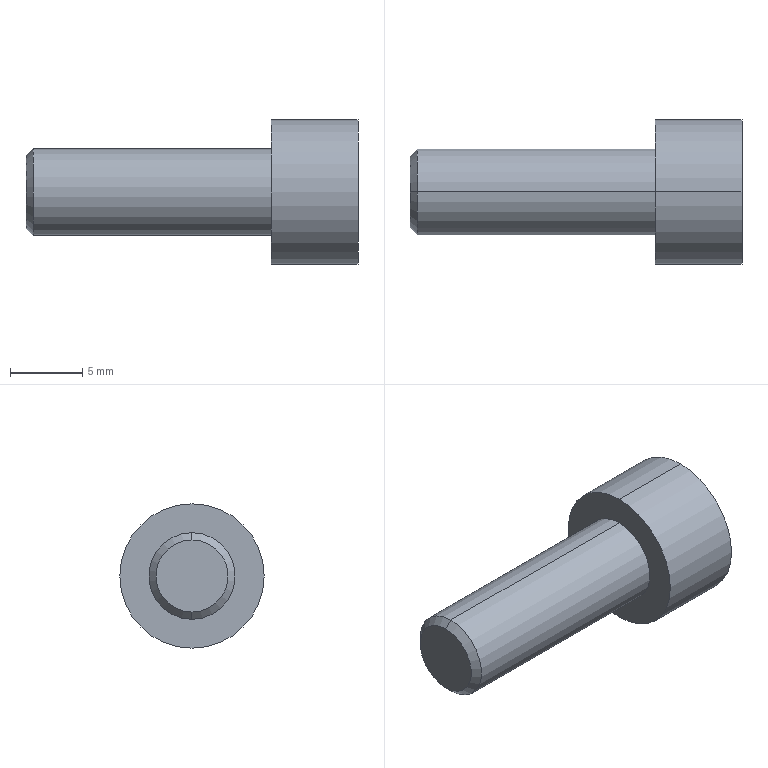Part | STEP file | 4-20.sldasm-Part-130 | 1 solid | 16 faces | box 23 x 10 x 10 mm | volume 863.941 mm3 | plane 10 | cylinder 4 | cone 2 | commonest cylinder face diameters 6 x2 10 x2
STEP:
#1=CARTESIAN_POINT('',(210.,264.383,-83.5));
#2=VERTEX_POINT('',#1);
#3=CARTESIAN_POINT('',(210.,264.383,-88.5));
#4=VERTEX_POINT('',#3);
#5=CARTESIAN_POINT('',(210.,264.383,-86.));
#6=DIRECTION('',(1.,0.,0.));
#7=DIRECTION('',(0.,-1.,0.));
#8=AXIS2_PLACEMENT_3D('',#5,#6,#7);
#9=CIRCLE('',#8,2.5);
#10=EDGE_CURVE('',#2,#4,#9,.T.);
#11=ORIENTED_EDGE('',*,*,#10,.T.);
#12=CARTESIAN_POINT('',(210.5,264.383,-89.));
#13=VERTEX_POINT('',#12);
#14=CARTESIAN_POINT('',(210.,264.383,-88.5));
#15=DIRECTION('',(0.7071,0.,-0.7071));
#16=VECTOR('',#15,1000.);
#17=LINE('',#14,#16);
#18=EDGE_CURVE('',#4,#13,#17,.T.);
#19=ORIENTED_EDGE('',*,*,#18,.T.);
#20=CARTESIAN_POINT('',(210.5,264.383,-83.));
#21=VERTEX_POINT('',#20);
#22=CARTESIAN_POINT('',(210.5,264.383,-86.));
#23=DIRECTION('',(-1.,0.,0.));
#24=DIRECTION('',(0.,0.,-1.));
#25=AXIS2_PLACEMENT_3D('',#22,#23,#24);
#26=CIRCLE('',#25,3.);
#27=EDGE_CURVE('',#13,#21,#26,.T.);
#28=ORIENTED_EDGE('',*,*,#27,.T.);
#29=CARTESIAN_POINT('',(210.,264.383,-83.5));
#30=DIRECTION('',(0.7071,0.,0.7071));
#31=VECTOR('',#30,1000.);
#32=LINE('',#29,#31);
#33=EDGE_CURVE('',#2,#21,#32,.T.);
#34=ORIENTED_EDGE('',*,*,#33,.F.);
#35=EDGE_LOOP('',(#11,#19,#28,#34));
#36=FACE_OUTER_BOUND('',#35,.T.);
#37=CARTESIAN_POINT('',(210.,264.383,-86.));
#38=DIRECTION('',(1.,0.,0.));
#39=DIRECTION('',(0.,0.,1.));
#40=AXIS2_PLACEMENT_3D('',#37,#38,#39);
#41=CONICAL_SURFACE('',#40,2.5,0.7854);
#42=ADVANCED_FACE('',(#36),#41,.T.);
#43=CARTESIAN_POINT('',(227.,264.383,-81.));
#44=VERTEX_POINT('',#43);
#45=CARTESIAN_POINT('',(227.,264.383,-91.));
#46=VERTEX_POINT('',#45);
#47=CARTESIAN_POINT('',(227.,264.383,-86.));
#48=DIRECTION('',(1.,0.,0.));
#49=DIRECTION('',(0.,0.,1.));
#50=AXIS2_PLACEMENT_3D('',#47,#48,#49);
#51=CIRCLE('',#50,5.);
#52=EDGE_CURVE('',#44,#46,#51,.T.);
#53=ORIENTED_EDGE('',*,*,#52,.T.);
#54=CARTESIAN_POINT('',(233.,264.383,-91.));
#55=VERTEX_POINT('',#54);
#56=CARTESIAN_POINT('',(227.,264.383,-91.));
#57=DIRECTION('',(1.,0.,0.));
#58=VECTOR('',#57,1000.);
#59=LINE('',#56,#58);
#60=EDGE_CURVE('',#46,#55,#59,.T.);
#61=ORIENTED_EDGE('',*,*,#60,.T.);
#62=CARTESIAN_POINT('',(233.,264.383,-81.));
#63=VERTEX_POINT('',#62);
#64=CARTESIAN_POINT('',(233.,264.383,-86.));
#65=DIRECTION('',(1.,0.,0.));
#66=DIRECTION('',(0.,0.,1.));
#67=AXIS2_PLACEMENT_3D('',#64,#65,#66);
#68=CIRCLE('',#67,5.);
#69=EDGE_CURVE('',#63,#55,#68,.T.);
#70=ORIENTED_EDGE('',*,*,#69,.F.);
#71=CARTESIAN_POINT('',(227.,264.383,-81.));
#72=DIRECTION('',(1.,0.,0.));
#73=VECTOR('',#72,1000.);
#74=LINE('',#71,#73);
#75=EDGE_CURVE('',#44,#63,#74,.T.);
#76=ORIENTED_EDGE('',*,*,#75,.F.);
#77=EDGE_LOOP('',(#53,#61,#70,#76));
#78=FACE_OUTER_BOUND('',#77,.T.);
#79=CARTESIAN_POINT('',(227.,264.383,-86.));
#80=DIRECTION('',(1.,0.,0.));
#81=DIRECTION('',(0.,0.,1.));
#82=AXIS2_PLACEMENT_3D('',#79,#80,#81);
#83=CYLINDRICAL_SURFACE('',#82,5.);
#84=ADVANCED_FACE('',(#78),#83,.T.);
#85=CARTESIAN_POINT('',(227.,264.383,-83.));
#86=VERTEX_POINT('',#85);
#87=CARTESIAN_POINT('',(227.,264.383,-89.));
#88=VERTEX_POINT('',#87);
#89=CARTESIAN_POINT('',(227.,264.383,-86.));
#90=DIRECTION('',(1.,0.,0.));
#91=DIRECTION('',(0.,0.,1.));
#92=AXIS2_PLACEMENT_3D('',#89,#90,#91);
#93=CIRCLE('',#92,3.);
#94=EDGE_CURVE('',#86,#88,#93,.T.);
#95=ORIENTED_EDGE('',*,*,#94,.F.);
#96=CARTESIAN_POINT('',(227.,264.383,-83.));
#97=DIRECTION('',(-1.,0.,0.));
#98=VECTOR('',#97,1000.);
#99=LINE('',#96,#98);
#100=EDGE_CURVE('',#86,#21,#99,.T.);
#101=ORIENTED_EDGE('',*,*,#100,.T.);
#102=ORIENTED_EDGE('',*,*,#27,.F.);
#103=CARTESIAN_POINT('',(227.,264.383,-89.));
#104=DIRECTION('',(-1.,0.,0.));
#105=VECTOR('',#104,1000.);
#106=LINE('',#103,#105);
#107=EDGE_CURVE('',#88,#13,#106,.T.);
#108=ORIENTED_EDGE('',*,*,#107,.F.);
#109=EDGE_LOOP('',(#95,#101,#102,#108));
#110=FACE_OUTER_BOUND('',#109,.T.);
#111=CARTESIAN_POINT('',(227.,264.383,-86.));
#112=DIRECTION('',(-1.,0.,0.));
#113=DIRECTION('',(0.,0.,-1.));
#114=AXIS2_PLACEMENT_3D('',#111,#112,#113);
#115=CYLINDRICAL_SURFACE('',#114,3.);
#116=ADVANCED_FACE('',(#110),#115,.T.);
#117=ORIENTED_EDGE('',*,*,#100,.F.);
#118=CARTESIAN_POINT('',(227.,264.383,-86.));
#119=DIRECTION('',(1.,0.,0.));
#120=DIRECTION('',(0.,0.,1.));
#121=AXIS2_PLACEMENT_3D('',#118,#119,#120);
#122=CIRCLE('',#121,3.);
#123=EDGE_CURVE('',#88,#86,#122,.T.);
#124=ORIENTED_EDGE('',*,*,#123,.F.);
#125=ORIENTED_EDGE('',*,*,#107,.T.);
#126=CARTESIAN_POINT('',(210.5,264.383,-86.));
#127=DIRECTION('',(-1.,0.,0.));
#128=DIRECTION('',(0.,0.,-1.));
#129=AXIS2_PLACEMENT_3D('',#126,#127,#128);
#130=CIRCLE('',#129,3.);
#131=EDGE_CURVE('',#21,#13,#130,.T.);
#132=ORIENTED_EDGE('',*,*,#131,.F.);
#133=EDGE_LOOP('',(#117,#124,#125,#132));
#134=FACE_OUTER_BOUND('',#133,.T.);
#135=CARTESIAN_POINT('',(227.,264.383,-86.));
#136=DIRECTION('',(-1.,0.,0.));
#137=DIRECTION('',(0.,0.,-1.));
#138=AXIS2_PLACEMENT_3D('',#135,#136,#137);
#139=CYLINDRICAL_SURFACE('',#138,3.);
#140=ADVANCED_FACE('',(#134),#139,.T.);
#141=ORIENTED_EDGE('',*,*,#52,.F.);
#142=CARTESIAN_POINT('',(227.,264.383,-86.));
#143=DIRECTION('',(1.,0.,0.));
#144=DIRECTION('',(0.,0.,1.));
#145=AXIS2_PLACEMENT_3D('',#142,#143,#144);
#146=CIRCLE('',#145,5.);
#147=EDGE_CURVE('',#46,#44,#146,.T.);
#148=ORIENTED_EDGE('',*,*,#147,.F.);
#149=EDGE_LOOP('',(#141,#148));
#150=FACE_OUTER_BOUND('',#149,.T.);
#151=ORIENTED_EDGE('',*,*,#123,.T.);
#152=ORIENTED_EDGE('',*,*,#94,.T.);
#153=EDGE_LOOP('',(#151,#152));
#154=FACE_BOUND('',#153,.T.);
#155=CARTESIAN_POINT('',(227.,264.383,-86.));
#156=DIRECTION('',(-1.,0.,0.));
#157=DIRECTION('',(0.,0.,-1.));
#158=AXIS2_PLACEMENT_3D('',#155,#156,#157);
#159=PLANE('',#158);
#160=ADVANCED_FACE('',(#150,#154),#159,.T.);
#161=CARTESIAN_POINT('',(233.,266.883,-87.443));
#162=VERTEX_POINT('',#161);
#163=CARTESIAN_POINT('',(233.,266.883,-84.557));
#164=VERTEX_POINT('',#163);
#165=CARTESIAN_POINT('',(233.,266.883,-87.443));
#166=DIRECTION('',(0.,0.,1.));
#167=VECTOR('',#166,1000.);
#168=LINE('',#165,#167);
#169=EDGE_CURVE('',#162,#164,#168,.T.);
#170=ORIENTED_EDGE('',*,*,#169,.F.);
#171=CARTESIAN_POINT('',(233.,264.383,-88.887));
#172=VERTEX_POINT('',#171);
#173=CARTESIAN_POINT('',(233.,264.383,-88.887));
#174=DIRECTION('',(0.,0.866,0.5));
#175=VECTOR('',#174,1000.);
#176=LINE('',#173,#175);
#177=EDGE_CURVE('',#172,#162,#176,.T.);
#178=ORIENTED_EDGE('',*,*,#177,.F.);
#179=CARTESIAN_POINT('',(233.,261.883,-87.443));
#180=VERTEX_POINT('',#179);
#181=CARTESIAN_POINT('',(233.,261.883,-87.443));
#182=DIRECTION('',(0.,0.866,-0.5));
#183=VECTOR('',#182,1000.);
#184=LINE('',#181,#183);
#185=EDGE_CURVE('',#180,#172,#184,.T.);
#186=ORIENTED_EDGE('',*,*,#185,.F.);
#187=CARTESIAN_POINT('',(233.,261.883,-84.557));
#188=VERTEX_POINT('',#187);
#189=CARTESIAN_POINT('',(233.,261.883,-84.557));
#190=DIRECTION('',(0.,0.,-1.));
#191=VECTOR('',#190,1000.);
#192=LINE('',#189,#191);
#193=EDGE_CURVE('',#188,#180,#192,.T.);
#194=ORIENTED_EDGE('',*,*,#193,.F.);
#195=CARTESIAN_POINT('',(233.,264.383,-83.113));
#196=VERTEX_POINT('',#195);
#197=CARTESIAN_POINT('',(233.,264.383,-83.113));
#198=DIRECTION('',(0.,-0.866,-0.5));
#199=VECTOR('',#198,1000.);
#200=LINE('',#197,#199);
#201=EDGE_CURVE('',#196,#188,#200,.T.);
#202=ORIENTED_EDGE('',*,*,#201,.F.);
#203=CARTESIAN_POINT('',(233.,266.883,-84.557));
#204=DIRECTION('',(0.,-0.866,0.5));
#205=VECTOR('',#204,1000.);
#206=LINE('',#203,#205);
#207=EDGE_CURVE('',#164,#196,#206,.T.);
#208=ORIENTED_EDGE('',*,*,#207,.F.);
#209=EDGE_LOOP('',(#170,#178,#186,#194,#202,#208));
#210=FACE_BOUND('',#209,.T.);
#211=ORIENTED_EDGE('',*,*,#69,.T.);
#212=CARTESIAN_POINT('',(233.,264.383,-86.));
#213=DIRECTION('',(1.,0.,0.));
#214=DIRECTION('',(0.,0.,1.));
#215=AXIS2_PLACEMENT_3D('',#212,#213,#214);
#216=CIRCLE('',#215,5.);
#217=EDGE_CURVE('',#55,#63,#216,.T.);
#218=ORIENTED_EDGE('',*,*,#217,.T.);
#219=EDGE_LOOP('',(#211,#218));
#220=FACE_OUTER_BOUND('',#219,.T.);
#221=CARTESIAN_POINT('',(233.,264.383,-86.));
#222=DIRECTION('',(1.,0.,0.));
#223=DIRECTION('',(0.,0.,1.));
#224=AXIS2_PLACEMENT_3D('',#221,#222,#223);
#225=PLANE('',#224);
#226=ADVANCED_FACE('',(#210,#220),#225,.T.);
#227=ORIENTED_EDGE('',*,*,#60,.F.);
#228=ORIENTED_EDGE('',*,*,#147,.T.);
#229=ORIENTED_EDGE('',*,*,#75,.T.);
#230=ORIENTED_EDGE('',*,*,#217,.F.);
#231=EDGE_LOOP('',(#227,#228,#229,#230));
#232=FACE_OUTER_BOUND('',#231,.T.);
#233=CARTESIAN_POINT('',(227.,264.383,-86.));
#234=DIRECTION('',(1.,0.,0.));
#235=DIRECTION('',(0.,0.,1.));
#236=AXIS2_PLACEMENT_3D('',#233,#234,#235);
#237=CYLINDRICAL_SURFACE('',#236,5.);
#238=ADVANCED_FACE('',(#232),#237,.T.);
#239=ORIENTED_EDGE('',*,*,#169,.T.);
#240=CARTESIAN_POINT('',(229.04,266.883,-84.557));
#241=VERTEX_POINT('',#240);
#242=CARTESIAN_POINT('',(229.04,266.883,-84.557));
#243=DIRECTION('',(1.,0.,0.));
#244=VECTOR('',#243,1000.);
#245=LINE('',#242,#244);
#246=EDGE_CURVE('',#241,#164,#245,.T.);
#247=ORIENTED_EDGE('',*,*,#246,.F.);
#248=CARTESIAN_POINT('',(229.04,266.883,-87.443));
#249=VERTEX_POINT('',#248);
#250=CARTESIAN_POINT('',(229.04,266.883,-87.443));
#251=DIRECTION('',(0.,0.,1.));
#252=VECTOR('',#251,1000.);
#253=LINE('',#250,#252);
#254=EDGE_CURVE('',#249,#241,#253,.T.);
#255=ORIENTED_EDGE('',*,*,#254,.F.);
#256=CARTESIAN_POINT('',(229.04,266.883,-87.443));
#257=DIRECTION('',(1.,0.,0.));
#258=VECTOR('',#257,1000.);
#259=LINE('',#256,#258);
#260=EDGE_CURVE('',#249,#162,#259,.T.);
#261=ORIENTED_EDGE('',*,*,#260,.T.);
#262=EDGE_LOOP('',(#239,#247,#255,#261));
#263=FACE_OUTER_BOUND('',#262,.T.);
#264=CARTESIAN_POINT('',(229.04,266.883,-87.443));
#265=DIRECTION('',(0.,1.,0.));
#266=DIRECTION('',(-1.,0.,0.));
#267=AXIS2_PLACEMENT_3D('',#264,#265,#266);
#268=PLANE('',#267);
#269=ADVANCED_FACE('',(#263),#268,.F.);
#270=ORIENTED_EDGE('',*,*,#207,.T.);
#271=CARTESIAN_POINT('',(229.04,264.383,-83.113));
#272=VERTEX_POINT('',#271);
#273=CARTESIAN_POINT('',(229.04,264.383,-83.113));
#274=DIRECTION('',(1.,0.,0.));
#275=VECTOR('',#274,1000.);
#276=LINE('',#273,#275);
#277=EDGE_CURVE('',#272,#196,#276,.T.);
#278=ORIENTED_EDGE('',*,*,#277,.F.);
#279=CARTESIAN_POINT('',(229.04,266.883,-84.557));
#280=DIRECTION('',(0.,-0.866,0.5));
#281=VECTOR('',#280,1000.);
#282=LINE('',#279,#281);
#283=EDGE_CURVE('',#241,#272,#282,.T.);
#284=ORIENTED_EDGE('',*,*,#283,.F.);
#285=ORIENTED_EDGE('',*,*,#246,.T.);
#286=EDGE_LOOP('',(#270,#278,#284,#285));
#287=FACE_OUTER_BOUND('',#286,.T.);
#288=CARTESIAN_POINT('',(229.04,266.883,-84.557));
#289=DIRECTION('',(0.,0.5,0.866));
#290=DIRECTION('',(0.,-0.866,0.5));
#291=AXIS2_PLACEMENT_3D('',#288,#289,#290);
#292=PLANE('',#291);
#293=ADVANCED_FACE('',(#287),#292,.F.);
#294=ORIENTED_EDGE('',*,*,#201,.T.);
#295=CARTESIAN_POINT('',(229.04,261.883,-84.557));
#296=VERTEX_POINT('',#295);
#297=CARTESIAN_POINT('',(229.04,261.883,-84.557));
#298=DIRECTION('',(1.,0.,0.));
#299=VECTOR('',#298,1000.);
#300=LINE('',#297,#299);
#301=EDGE_CURVE('',#296,#188,#300,.T.);
#302=ORIENTED_EDGE('',*,*,#301,.F.);
#303=CARTESIAN_POINT('',(229.04,264.383,-83.113));
#304=DIRECTION('',(0.,-0.866,-0.5));
#305=VECTOR('',#304,1000.);
#306=LINE('',#303,#305);
#307=EDGE_CURVE('',#272,#296,#306,.T.);
#308=ORIENTED_EDGE('',*,*,#307,.F.);
#309=ORIENTED_EDGE('',*,*,#277,.T.);
#310=EDGE_LOOP('',(#294,#302,#308,#309));
#311=FACE_OUTER_BOUND('',#310,.T.);
#312=CARTESIAN_POINT('',(229.04,264.383,-83.113));
#313=DIRECTION('',(0.,-0.5,0.866));
#314=DIRECTION('',(0.,-0.866,-0.5));
#315=AXIS2_PLACEMENT_3D('',#312,#313,#314);
#316=PLANE('',#315);
#317=ADVANCED_FACE('',(#311),#316,.F.);
#318=ORIENTED_EDGE('',*,*,#193,.T.);
#319=CARTESIAN_POINT('',(229.04,261.883,-87.443));
#320=VERTEX_POINT('',#319);
#321=CARTESIAN_POINT('',(229.04,261.883,-87.443));
#322=DIRECTION('',(1.,0.,0.));
#323=VECTOR('',#322,1000.);
#324=LINE('',#321,#323);
#325=EDGE_CURVE('',#320,#180,#324,.T.);
#326=ORIENTED_EDGE('',*,*,#325,.F.);
#327=CARTESIAN_POINT('',(229.04,261.883,-84.557));
#328=DIRECTION('',(0.,0.,-1.));
#329=VECTOR('',#328,1000.);
#330=LINE('',#327,#329);
#331=EDGE_CURVE('',#296,#320,#330,.T.);
#332=ORIENTED_EDGE('',*,*,#331,.F.);
#333=ORIENTED_EDGE('',*,*,#301,.T.);
#334=EDGE_LOOP('',(#318,#326,#332,#333));
#335=FACE_OUTER_BOUND('',#334,.T.);
#336=CARTESIAN_POINT('',(229.04,261.883,-84.557));
#337=DIRECTION('',(0.,-1.,0.));
#338=DIRECTION('',(1.,0.,0.));
#339=AXIS2_PLACEMENT_3D('',#336,#337,#338);
#340=PLANE('',#339);
#341=ADVANCED_FACE('',(#335),#340,.F.);
#342=ORIENTED_EDGE('',*,*,#185,.T.);
#343=CARTESIAN_POINT('',(229.04,264.383,-88.887));
#344=VERTEX_POINT('',#343);
#345=CARTESIAN_POINT('',(229.04,264.383,-88.887));
#346=DIRECTION('',(1.,0.,0.));
#347=VECTOR('',#346,1000.);
#348=LINE('',#345,#347);
#349=EDGE_CURVE('',#344,#172,#348,.T.);
#350=ORIENTED_EDGE('',*,*,#349,.F.);
#351=CARTESIAN_POINT('',(229.04,261.883,-87.443));
#352=DIRECTION('',(0.,0.866,-0.5));
#353=VECTOR('',#352,1000.);
#354=LINE('',#351,#353);
#355=EDGE_CURVE('',#320,#344,#354,.T.);
#356=ORIENTED_EDGE('',*,*,#355,.F.);
#357=ORIENTED_EDGE('',*,*,#325,.T.);
#358=EDGE_LOOP('',(#342,#350,#356,#357));
#359=FACE_OUTER_BOUND('',#358,.T.);
#360=CARTESIAN_POINT('',(229.04,261.883,-87.443));
#361=DIRECTION('',(0.,-0.5,-0.866));
#362=DIRECTION('',(0.,0.866,-0.5));
#363=AXIS2_PLACEMENT_3D('',#360,#361,#362);
#364=PLANE('',#363);
#365=ADVANCED_FACE('',(#359),#364,.F.);
#366=ORIENTED_EDGE('',*,*,#177,.T.);
#367=ORIENTED_EDGE('',*,*,#260,.F.);
#368=CARTESIAN_POINT('',(229.04,264.383,-88.887));
#369=DIRECTION('',(0.,0.866,0.5));
#370=VECTOR('',#369,1000.);
#371=LINE('',#368,#370);
#372=EDGE_CURVE('',#344,#249,#371,.T.);
#373=ORIENTED_EDGE('',*,*,#372,.F.);
#374=ORIENTED_EDGE('',*,*,#349,.T.);
#375=EDGE_LOOP('',(#366,#367,#373,#374));
#376=FACE_OUTER_BOUND('',#375,.T.);
#377=CARTESIAN_POINT('',(229.04,264.383,-88.887));
#378=DIRECTION('',(0.,0.5,-0.866));
#379=DIRECTION('',(0.,0.866,0.5));
#380=AXIS2_PLACEMENT_3D('',#377,#378,#379);
#381=PLANE('',#380);
#382=ADVANCED_FACE('',(#376),#381,.F.);
#383=ORIENTED_EDGE('',*,*,#254,.T.);
#384=ORIENTED_EDGE('',*,*,#283,.T.);
#385=ORIENTED_EDGE('',*,*,#307,.T.);
#386=ORIENTED_EDGE('',*,*,#331,.T.);
#387=ORIENTED_EDGE('',*,*,#355,.T.);
#388=ORIENTED_EDGE('',*,*,#372,.T.);
#389=EDGE_LOOP('',(#383,#384,#385,#386,#387,#388));
#390=FACE_OUTER_BOUND('',#389,.T.);
#391=CARTESIAN_POINT('',(229.04,266.883,-84.557));
#392=DIRECTION('',(1.,0.,0.));
#393=DIRECTION('',(0.,0.,1.));
#394=AXIS2_PLACEMENT_3D('',#391,#392,#393);
#395=PLANE('',#394);
#396=ADVANCED_FACE('',(#390),#395,.T.);
#397=ORIENTED_EDGE('',*,*,#10,.F.);
#398=CARTESIAN_POINT('',(210.,264.383,-86.));
#399=DIRECTION('',(1.,0.,0.));
#400=DIRECTION('',(0.,-1.,0.));
#401=AXIS2_PLACEMENT_3D('',#398,#399,#400);
#402=CIRCLE('',#401,2.5);
#403=EDGE_CURVE('',#4,#2,#402,.T.);
#404=ORIENTED_EDGE('',*,*,#403,.F.);
#405=EDGE_LOOP('',(#397,#404));
#406=FACE_OUTER_BOUND('',#405,.T.);
#407=CARTESIAN_POINT('',(210.,330.383,-68.));
#408=DIRECTION('',(-1.,0.,0.));
#409=DIRECTION('',(0.,-1.,0.));
#410=AXIS2_PLACEMENT_3D('',#407,#408,#409);
#411=PLANE('',#410);
#412=ADVANCED_FACE('',(#406),#411,.T.);
#413=ORIENTED_EDGE('',*,*,#18,.F.);
#414=ORIENTED_EDGE('',*,*,#403,.T.);
#415=ORIENTED_EDGE('',*,*,#33,.T.);
#416=ORIENTED_EDGE('',*,*,#131,.T.);
#417=EDGE_LOOP('',(#413,#414,#415,#416));
#418=FACE_OUTER_BOUND('',#417,.T.);
#419=CARTESIAN_POINT('',(210.,264.383,-86.));
#420=DIRECTION('',(1.,0.,0.));
#421=DIRECTION('',(0.,0.,1.));
#422=AXIS2_PLACEMENT_3D('',#419,#420,#421);
#423=CONICAL_SURFACE('',#422,2.5,0.7854);
#424=ADVANCED_FACE('',(#418),#423,.T.);
#425=CLOSED_SHELL('',(#42,#84,#116,#140,#160,#226,#238,#269,#293,#317,#341,#365,#382,#396,#412,#424));
#426=MANIFOLD_SOLID_BREP('',#425);
#427=CARTESIAN_POINT('',(0.,0.,0.));
#428=DIRECTION('',(0.,0.,1.));
#429=DIRECTION('',(1.,0.,0.));
#430=AXIS2_PLACEMENT_3D('',#427,#428,#429);
#431=(LENGTH_UNIT()NAMED_UNIT(*)SI_UNIT(.MILLI.,.METRE.));
#432=UNCERTAINTY_MEASURE_WITH_UNIT(LENGTH_MEASURE(0.00001),#431,'','');
#433=(NAMED_UNIT(*)PLANE_ANGLE_UNIT()SI_UNIT($,.RADIAN.));
#434=(NAMED_UNIT(*)SI_UNIT($,.STERADIAN.)SOLID_ANGLE_UNIT());
#435=(GEOMETRIC_REPRESENTATION_CONTEXT(3)GLOBAL_UNCERTAINTY_ASSIGNED_CONTEXT((#432))GLOBAL_UNIT_ASSIGNED_CONTEXT((#431,#433,#434))REPRESENTATION_CONTEXT('',''));
#436=ADVANCED_BREP_SHAPE_REPRESENTATION('',(#426,#430),#435);